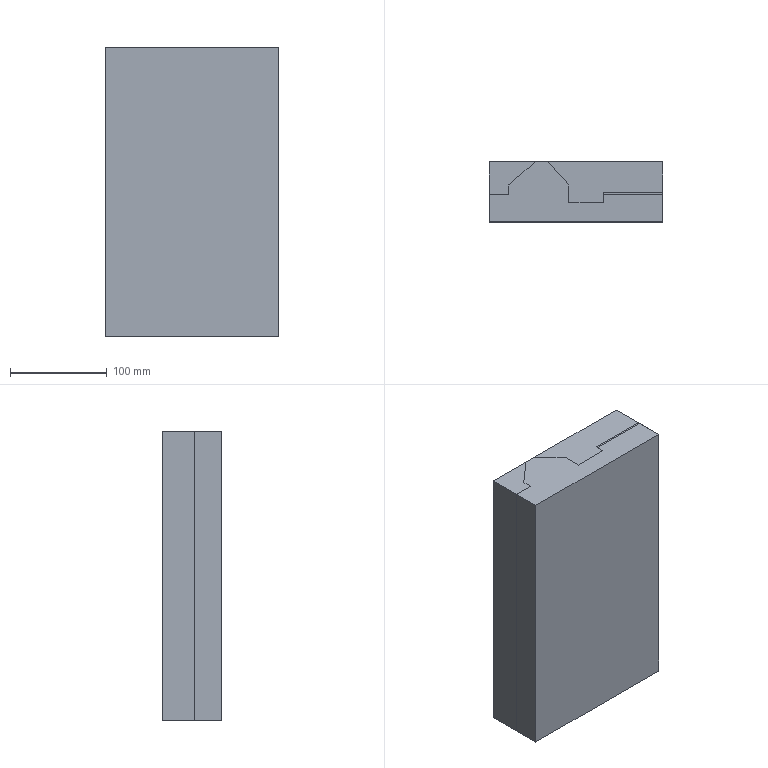NC program | NX | posted with a generic post | part box 180 x 62 x 300 mm
Lines 1 to 1029 of 29776:
N10 G17 G21 G94 G90
(型腔铣_COPY , TOOL : D50飞刀)
N12 T14 M6
N14 /M1
N16 G54
N18 G17 G0 G90 X-218.484 Y125.131 S1500 M3
N20 G43 Z20. H14
N22 Z-9.3
N24 G94 G1 Z-10.3 F2000.
N26 G3 X-181.258 Y93.895 R37.8
N28 G1 X-152.134
N30 G2 X-150. Y93.915 R113.9
N32 G1 X150.
N34 G2 X152.134 Y93.895 R113.9
N36 G1 X175.831
N38 G2 X179.344 Y92.674 R5.67 F1880.
N40 X181.345 Y89.54 R5.67 F1760.
N42 X181.5 Y88.226 R5.67 F1640.
N44 G1 Y85.763
N46 Y81.975 F1520.
N48 Y78.186 F1400.
N50 Y74.397 F1280.
N52 Y70.608 F1160.
N54 Y66.819 F1040.
N56 Y63.03 F920.
N58 Y59.242 F800.
N60 G2 X175.203 Y52.945 R6.3
N62 G1 X151.708 F2000.
N64 G3 X150. Y52.965 R72.95
N66 G1 X-150.
N68 G3 X-151.708 Y52.945 R72.95
N70 G1 X-175.201
N72 G3 X-178.934 Y51.719 R6.3 F1880.
N74 X-181.214 Y48.52 R6.3 F1760.
N76 X-181.5 Y46.646 R6.3 F1640.
N78 G1 Y44.554
N80 Y40.559 F1520.
N82 Y36.564 F1400.
N84 Y32.569 F1280.
N86 Y28.574 F1160.
N88 Y24.741 F1040.
N90 Y24.579
N92 Y24.496 F920.
N94 X-183.176 Y20.962
N96 X-184.888 Y17.352 F800.
N98 G3 X-181.5 Y11.995 R3.75
N100 G1 X-168.9
N102 X-156.3 F1040.
N104 X-151.131 F1280.
N106 G2 X-150. Y12.015 R32.
N108 G1 X-143.7
N110 X-131.1 F1520.
N112 X-118.5 F1760.
N114 X150. F2000.
N116 G2 X151.131 Y11.995 R32.
N118 G1 X181.5
N120 G3 X194.1 Y15.371 R25.2
N122 G0 Z20.
N124 X-218.449 Y125.404
N126 Z-9.6
N128 G1 Z-10.6
N130 G3 X-181.223 Y94.168 R37.8
N132 G1 X-152.129
N134 G2 X-150.013 Y94.188 R113.905
N136 G1 X150.
N138 G2 X152.134 Y94.168 R113.9
N140 G1 X175.831
N142 G2 X179.344 Y92.948 R5.67 F1880.
N144 X181.345 Y89.813 R5.67 F1760.
N146 X181.5 Y88.499 R5.67 F1640.
N148 G1 Y86.037
N150 Y82.248 F1520.
N152 Y78.459 F1400.
N154 Y74.67 F1280.
N156 Y70.881 F1160.
N158 Y67.092 F1040.
N160 Y63.304 F920.
N162 Y59.515 F800.
N164 G2 X175.203 Y53.218 R6.3
N166 G1 X151.708 F2000.
N168 G3 X150. Y53.238 R72.95
N170 G1 X-150.007
N172 G3 X-151.703 Y53.218 R72.955
N174 G1 X-175.201
N176 G3 X-178.942 Y51.987 R6.3 F1880.
N178 X-181.22 Y48.775 R6.3 F1760.
N180 X-181.5 Y46.919 R6.3 F1640.
N182 G1 Y44.798
N184 Y40.793 F1520.
N186 Y36.788 F1400.
N188 Y32.782 F1280.
N190 Y28.777 F1160.
N192 Y24.741 F1040.
N194 Y24.496 F920.
N196 X-183.098 Y21.127
N198 X-184.814 Y17.508 F800.
N200 G3 X-181.5 Y12.268 R3.668
N202 G1 X-168.9
N204 X-156.3 F1040.
N206 X-151.126 F1280.
N208 G2 X-150. Y12.288 R32.005
N210 G1 X-143.7
N212 X-131.1 F1520.
N214 X-118.5 F1760.
N216 X150. F2000.
N218 G2 X151.131 Y12.268 R32.
N220 G1 X181.5
N222 G3 X194.1 Y15.644 R25.2
N224 G0 Z20.
N226 X-218.411 Y125.678
N228 Z-9.9
N230 G1 Z-10.9
N232 G3 X-181.185 Y94.441 R37.8
N234 G1 X-152.134
N236 G2 X-150. Y94.461 R113.9
N238 G1 X150.
N240 G2 X152.134 Y94.441 R113.9
N242 G1 X175.831
N244 G2 X179.344 Y93.221 R5.67 F1880.
N246 X181.345 Y90.087 R5.67 F1760.
N248 X181.5 Y88.773 R5.67 F1640.
N250 G1 Y86.31
N252 Y82.521 F1520.
N254 Y78.733 F1400.
N256 Y74.944 F1280.
N258 Y71.155 F1160.
N260 Y67.366 F1040.
N262 Y63.577 F920.
N264 Y59.788 F800.
N266 G2 X175.203 Y53.491 R6.3
N268 G1 X151.708 F2000.
N270 G3 X150. Y53.511 R72.95
N272 G1 X-150.
N274 G3 X-151.708 Y53.491 R72.95
N276 G1 X-175.201
N278 G3 X-178.95 Y52.254 R6.3 F1880.
N280 X-181.226 Y49.029 R6.3 F1760.
N282 X-181.5 Y47.193 R6.3 F1640.
N284 G1 Y45.041
N286 Y41.026 F1520.
N288 Y37.011 F1400.
N290 Y32.996 F1280.
N292 Y28.98 F1160.
N294 Y24.965 F1040.
N296 Y24.741 F920.
N298 Y24.496
N300 X-183.019 Y21.292
N302 X-184.74 Y17.665 F800.
N304 G3 X-181.5 Y12.541 R3.586
N306 G1 X-168.9
N308 X-156.3 F1040.
N310 X-151.131 F1280.
N312 G2 X-150. Y12.561 R32.
N314 G1 X-143.7
N316 X-131.1 F1520.
N318 X-118.5 F1760.
N320 X150. F2000.
N322 G2 X151.131 Y12.541 R32.
N324 G1 X181.5
N326 G3 X194.1 Y15.918 R25.2
N328 G0 Z20.
N330 X-218.371 Y125.951
N332 Z-10.2
N334 G1 Z-11.2
N336 G3 X-181.145 Y94.715 R37.8
N338 G1 X-152.134
N340 G2 X-150. Y94.735 R113.9
N342 G1 X150.
N344 G2 X152.134 Y94.715 R113.9
N346 G1 X175.831
N348 G2 X179.344 Y93.495 R5.67 F1880.
N350 X181.345 Y90.36 R5.67 F1760.
N352 X181.5 Y89.046 R5.67 F1640.
N354 G1 Y86.584
N356 Y82.795 F1520.
N358 Y79.006 F1400.
N360 Y75.217 F1280.
N362 Y71.428 F1160.
N364 Y67.639 F1040.
N366 Y63.851 F920.
N368 Y60.062 F800.
N370 G2 X175.203 Y53.765 R6.3
N372 G1 X151.708 F2000.
N374 G3 X150. Y53.785 R72.95
N376 G1 X-150.
N378 G3 X-151.708 Y53.765 R72.95
N380 G1 X-175.201
N382 G3 X-178.958 Y52.521 R6.3 F1880.
N384 X-181.232 Y49.283 R6.3 F1760.
N386 X-181.5 Y47.466 R6.3 F1640.
N388 G1 Y45.284
N390 Y41.259 F1520.
N392 Y37.234 F1400.
N394 Y33.209 F1280.
N396 Y29.184 F1160.
N398 Y25.158 F1040.
N400 Y24.741 F920.
N402 Y24.496
N404 X-182.941 Y21.458
N406 X-184.666 Y17.821 F800.
N408 G3 X-181.5 Y12.815 R3.504
N410 G1 X-168.9
N412 X-156.3 F1040.
N414 X-151.131 F1280.
N416 G2 X-150. Y12.835 R32.
N418 G1 X-143.7
N420 X-131.1 F1520.
N422 X-118.5 F1760.
N424 X150. F2000.
N426 G2 X151.131 Y12.815 R32.
N428 G1 X181.5
N430 G3 X194.1 Y16.191 R25.2
N432 G0 Z20.
N434 X-218.328 Y126.224
N436 Z-10.5
N438 G1 Z-11.5
N440 G3 X-181.103 Y94.988 R37.8
N442 G1 X-152.134
N444 G2 X-150. Y95.008 R113.9
N446 G1 X150.
N448 G2 X152.134 Y94.988 R113.9
N450 G1 X175.831
N452 G2 X179.344 Y93.768 R5.67 F1880.
N454 X181.345 Y90.634 R5.67 F1760.
N456 X181.5 Y89.32 R5.67 F1640.
N458 G1 Y86.857
N460 Y83.068 F1520.
N462 Y79.279 F1400.
N464 Y75.491 F1280.
N466 Y71.702 F1160.
N468 Y67.913 F1040.
N470 Y64.124 F920.
N472 Y60.335 F800.
N474 G2 X175.203 Y54.038 R6.3
N476 G1 X151.708 F2000.
N478 G3 X150. Y54.058 R72.95
N480 G1 X-150.
N482 G3 X-151.708 Y54.038 R72.95
N484 G1 X-175.201
N486 G3 X-178.966 Y52.789 R6.3 F1880.
N488 X-181.238 Y49.537 R6.3 F1760.
N490 X-181.5 Y47.739 R6.3 F1640.
N492 G1 Y45.527
N494 Y41.492 F1520.
N496 Y37.457 F1400.
N498 Y33.422 F1280.
N500 Y29.387 F1160.
N502 Y25.351 F1040.
N504 Y24.741 F920.
N506 Y24.496
N508 X-182.863 Y21.623
N510 X-184.592 Y17.977 F800.
N512 G3 X-181.5 Y13.088 R3.422
N514 G1 X-168.9
N516 X-156.3 F1040.
N518 X-151.131 F1280.
N520 G2 X-150. Y13.108 R32.
N522 G1 X-143.7
N524 X-131.1 F1520.
N526 X-118.5 F1760.
N528 X150. F2000.
N530 G2 X151.131 Y13.088 R32.
N532 G1 X181.5
N534 G3 X194.1 Y16.464 R25.2
N536 G0 Z20.
N538 X-218.283 Y126.498
N540 Z-10.8
N542 G1 Z-11.8
N544 G3 X-181.057 Y95.262 R37.8
N546 G1 X-152.134
N548 G2 X-150. Y95.282 R113.9
N550 G1 X150.
N552 G2 X152.134 Y95.262 R113.9
N554 G1 X175.831
N556 G2 X179.344 Y94.041 R5.67 F1880.
N558 X181.345 Y90.907 R5.67 F1760.
N560 X181.5 Y89.593 R5.67 F1640.
N562 G1 Y87.13
N564 Y83.342 F1520.
N566 Y79.553 F1400.
N568 Y75.764 F1280.
N570 Y71.975 F1160.
N572 Y68.186 F1040.
N574 Y64.397 F920.
N576 Y60.609 F800.
N578 G2 X175.204 Y54.312 R6.3
N580 G1 X151.708 F2000.
N582 G3 X150. Y54.332 R72.95
N584 G1 X-150.
N586 G3 X-151.708 Y54.312 R72.95
N588 G1 X-175.201
N590 G3 X-178.974 Y53.056 R6.3 F1880.
N592 X-181.243 Y49.791 R6.3 F1760.
N594 X-181.5 Y48.013 R6.3 F1640.
N596 G1 Y45.771
N598 Y41.725 F1520.
N600 Y37.68 F1400.
N602 Y33.635 F1280.
N604 Y29.59 F1160.
N606 Y25.544 F1040.
N608 Y24.741 F920.
N610 Y24.496
N612 X-182.784 Y21.788
N614 X-184.518 Y18.133 F800.
N616 G3 X-181.5 Y13.362 R3.34
N618 G1 X-168.9
N620 X-156.3 F1040.
N622 X-151.131 F1280.
N624 G2 X-150. Y13.382 R32.
N626 G1 X-143.7
N628 X-131.1 F1520.
N630 X-118.5 F1760.
N632 X150. F2000.
N634 G2 X151.131 Y13.362 R32.
N636 G1 X181.5
N638 G3 X194.1 Y16.738 R25.2
N640 G0 Z20.
N642 X-218.236 Y126.771
N644 Z-11.1
N646 G1 Z-12.1
N648 G3 X-181.01 Y95.535 R37.8
N650 G1 X-152.13
N652 G2 X-150.012 Y95.555 R113.905
N654 G1 X150.
N656 G2 X152.134 Y95.535 R113.9
N658 G1 X175.831
N660 G2 X179.344 Y94.315 R5.67 F1880.
N662 X181.345 Y91.181 R5.67 F1760.
N664 X181.5 Y89.866 R5.67 F1640.
N666 G1 Y87.404
N668 Y83.615 F1520.
N670 Y79.826 F1400.
N672 Y76.037 F1280.
N674 Y72.248 F1160.
N676 Y68.46 F1040.
N678 Y64.671 F920.
N680 Y60.882 F800.
N682 G2 X175.203 Y54.585 R6.3
N684 G1 X151.708 F2000.
N686 G3 X150. Y54.605 R72.95
N688 G1 X-150.006
N690 G3 X-151.704 Y54.585 R72.955
N692 G1 X-175.201
N694 G3 X-178.982 Y53.324 R6.3 F1880.
N696 X-181.249 Y50.045 R6.3 F1760.
N698 X-181.5 Y48.286 R6.3 F1640.
N700 G1 Y46.014
N702 Y41.959 F1520.
N704 Y37.903 F1400.
N706 Y33.848 F1280.
N708 Y29.793 F1160.
N710 Y25.737 F1040.
N712 Y24.741 F920.
N714 Y24.496
N716 X-182.706 Y21.954
N718 X-184.444 Y18.289 F800.
N720 G3 X-181.5 Y13.635 R3.258
N722 G1 X-168.9
N724 X-156.3 F1040.
N726 X-151.127 F1280.
N728 G2 X-150. Y13.655 R32.005
N730 G1 X-143.7
N732 X-131.1 F1520.
N734 X-118.5 F1760.
N736 X150. F2000.
N738 G2 X151.131 Y13.635 R32.
N740 G1 X181.5
N742 G3 X194.1 Y17.011 R25.2
N744 G0 Z20.
N746 X-218.186 Y127.045
N748 Z-11.4
N750 G1 Z-12.4
N752 G3 X-180.96 Y95.808 R37.8
N754 G1 X-152.134
N756 G2 X-150. Y95.828 R113.9
N758 G1 X150.
N760 G2 X152.134 Y95.808 R113.9
N762 G1 X175.831
N764 G2 X179.344 Y94.588 R5.67 F1880.
N766 X181.345 Y91.454 R5.67 F1760.
N768 X181.5 Y90.17 R5.67 F1640.
N770 G1 Y90.
N772 Y87.677
N774 Y83.888 F1520.
N776 Y80.1 F1400.
N778 Y76.311 F1280.
N780 Y72.522 F1160.
N782 Y68.733 F1040.
N784 Y64.944 F920.
N786 Y61.155 F800.
N788 G2 X175.203 Y54.858 R6.3
N790 G1 X151.708 F2000.
N792 G3 X150. Y54.878 R72.95
N794 G1 X-150.
N796 G3 X-151.708 Y54.858 R72.95
N798 G1 X-175.201
N800 G3 X-178.99 Y53.591 R6.3 F1880.
N802 X-181.255 Y50.3 R6.3 F1760.
N804 X-181.5 Y48.56 R6.3 F1640.
N806 G1 Y46.257
N808 Y42.192 F1520.
N810 Y38.126 F1400.
N812 Y34.061 F1280.
N814 Y29.996 F1160.
N816 Y25.93 F1040.
N818 Y24.741 F920.
N820 Y24.496
N822 X-182.627 Y22.119
N824 X-184.369 Y18.446 F800.
N826 G3 X-181.5 Y13.908 R3.176
N828 G1 X-168.9
N830 X-156.3 F1040.
N832 X-151.131 F1280.
N834 G2 X-150. Y13.928 R32.
N836 G1 X-143.7
N838 X-131.1 F1520.
N840 X-118.5 F1760.
N842 X150. F2000.
N844 G2 X151.131 Y13.908 R32.
N846 G1 X181.5
N848 G3 X194.1 Y17.285 R25.2
N850 G0 Z20.
N852 X-218.133 Y127.318
N854 Z-11.7
N856 G1 Z-12.7
N858 G3 X-180.907 Y96.082 R37.8
N860 G1 X-152.134
N862 G2 X-150. Y96.102 R113.9
N864 G1 X150.
N866 G2 X152.134 Y96.082 R113.9
N868 G1 X175.828
N870 G2 X179.341 Y94.862 R5.67 F1880.
N872 X181.342 Y91.727 R5.67 F1760.
N874 X181.496 Y90.504 R5.67 F1640.
N876 X181.5 Y90. R31.5
N878 G1 Y87.951
N880 Y84.162 F1520.
N882 Y80.373 F1400.
N884 Y76.584 F1280.
N886 Y72.795 F1160.
N888 Y69.006 F1040.
N890 Y65.218 F920.
N892 Y61.429 F800.
N894 G2 X175.203 Y55.132 R6.3
N896 G1 X151.708 F2000.
N898 G3 X150. Y55.152 R72.95
N900 G1 X-150.
N902 G3 X-151.708 Y55.132 R72.95
N904 G1 X-175.201
N906 G3 X-178.998 Y53.858 R6.3 F1880.
N908 X-181.26 Y50.554 R6.3 F1760.
N910 X-181.5 Y48.833 R6.3 F1640.
N912 G1 Y46.5
N914 Y42.425 F1520.
N916 Y38.35 F1400.
N918 Y34.274 F1280.
N920 Y30.199 F1160.
N922 Y26.123 F1040.
N924 Y24.741 F920.
N926 Y24.496
N928 X-182.549 Y22.284
N930 X-184.295 Y18.602 F800.
N932 G3 X-181.5 Y14.182 R3.094
N934 G1 X-168.9
N936 X-156.3 F1040.
N938 X-151.131 F1280.
N940 G2 X-150. Y14.202 R32.
N942 G1 X-143.7
N944 X-131.1 F1520.
N946 X-118.5 F1760.
N948 X150. F2000.
N950 G2 X151.131 Y14.182 R32.
N952 G1 X181.5
N954 G3 X194.1 Y17.558 R25.2
N956 G0 Z20.
N958 X-218.078 Y127.591
N960 Z-12.
N962 G1 Z-13.
N964 G3 X-180.852 Y96.355 R37.8
N966 G1 X-152.134
N968 G2 X-150. Y96.375 R113.9
N970 G1 X150.
N972 G2 X152.134 Y96.355 R113.9
N974 G1 X175.822
N976 G2 X179.335 Y95.135 R5.67 F1880.
N978 X181.336 Y92.001 R5.67 F1760.
N980 X181.489 Y90.837 R5.67 F1640.
N982 X181.5 Y90. R31.5
N984 G1 Y88.224
N986 Y84.435 F1520.
N988 Y80.646 F1400.
N990 Y76.858 F1280.
N992 Y73.069 F1160.
N994 Y69.28 F1040.
N996 Y65.491 F920.
N998 Y61.702 F800.
N1000 G2 X175.204 Y55.405 R6.3
N1002 G1 X151.708 F2000.
N1004 G3 X150. Y55.425 R72.95
N1006 G1 X-150.
N1008 G3 X-151.708 Y55.405 R72.95
N1010 G1 X-175.201
N1012 G3 X-179.006 Y54.126 R6.3 F1880.
N1014 X-181.266 Y50.808 R6.3 F1760.
N1016 X-181.5 Y49.107 R6.3 F1640.
N1018 G1 Y46.744
N1020 Y42.658 F1520.
N1022 Y38.573 F1400.
N1024 Y34.487 F1280.
N1026 Y30.402 F1160.
N1028 Y26.316 F1040.
N1030 Y24.741 F920.
N1032 Y24.496
N1034 X-182.47 Y22.449
N1036 X-184.221 Y18.758 F800.
N1038 G3 X-181.5 Y14.455 R3.012
N1040 G1 X-168.9
N1042 X-156.3 F1040.
N1044 X-151.131 F1280.
N1046 G2 X-150. Y14.475 R32.
N1048 G1 X-143.7
N1050 X-131.1 F1520.
N1052 X-118.5 F1760.
N1054 X150. F2000.
N1056 G2 X151.131 Y14.455 R32.
N1058 G1 X181.5
N1060 G3 X194.1 Y17.831 R25.2
N1062 G0 Z20.
N1064 X-218.02 Y127.865
N1066 Z-12.3
N1068 G1 Z-13.3
N1070 G3 X-180.795 Y96.629 R37.8
N1072 G1 X-152.134
N1074 G2 X-150. Y96.649 R113.9
N1076 G1 X150.
N1078 G2 X152.134 Y96.629 R113.9
N1080 G1 X175.199
N1082 G2 X178.793 Y95.502 R6.3 F1880.
N1084 X181.102 Y92.527 R6.3 F1760.
N1086 X181.497 Y90.412 R6.3 F1640.
N1088 X181.5 Y90. R31.5
N1090 G1 Y88.749
N1092 Y84.924 F1520.
N1094 Y81.1 F1400.
N1096 Y77.275 F1280.
N1098 Y73.45 F1160.
N1100 Y69.625 F1040.
N1102 Y65.8 F920.
N1104 Y61.976 F800.
N1106 G2 X175.203 Y55.679 R6.3
N1108 G1 X151.708 F2000.
N1110 G3 X150. Y55.699 R72.95
N1112 G1 X-150.
N1114 G3 X-151.708 Y55.679 R72.95
N1116 G1 X-175.201
N1118 G3 X-179.014 Y54.393 R6.3 F1880.
N1120 X-181.271 Y51.062 R6.3 F1760.
N1122 X-181.5 Y49.38 R6.3 F1640.
N1124 G1 Y46.987
N1126 Y42.891 F1520.
N1128 Y38.796 F1400.
N1130 Y34.7 F1280.
N1132 Y30.605 F1160.
N1134 Y26.509 F1040.
N1136 Y24.741 F920.
N1138 Y24.496
N1140 X-182.392 Y22.615
N1142 X-184.147 Y18.914 F800.
N1144 G3 X-181.5 Y14.729 R2.93
N1146 G1 X-168.9
N1148 X-156.3 F1040.
N1150 X-151.131 F1280.
N1152 G2 X-150. Y14.749 R32.
N1154 G1 X-143.7
N1156 X-131.1 F1520.
N1158 X-118.5 F1760.
N1160 X150. F2000.
N1162 G2 X151.131 Y14.729 R32.
N1164 G1 X181.5
N1166 G3 X194.1 Y18.105 R25.2
N1168 G0 Z20.
N1170 X-217.96 Y128.138
N1172 Z-12.6
N1174 G1 Z-13.6
N1176 G3 X-180.735 Y96.902 R37.8
N1178 G1 X-152.134
N1180 G2 X-150. Y96.922 R113.9
N1182 G1 X150.
N1184 G2 X152.134 Y96.902 R113.9
N1186 G1 X175.194
N1188 G2 X178.788 Y95.776 R6.3 F1880.
N1190 X181.097 Y92.8 R6.3 F1760.
N1192 X181.491 Y90.754 R6.3 F1640.
N1194 X181.5 Y90. R31.5
N1196 G1 Y89.918
N1198 Y89.023
N1200 Y85.198 F1520.
N1202 Y81.373 F1400.
N1204 Y77.548 F1280.
N1206 Y73.723 F1160.
N1208 Y69.899 F1040.
N1210 Y66.074 F920.
N1212 Y62.249 F800.
N1214 G2 X175.203 Y55.952 R6.3
N1216 G1 X151.708 F2000.
N1218 G3 X150. Y55.972 R72.95
N1220 G1 X-150.
N1222 G3 X-151.708 Y55.952 R72.95
N1224 G1 X-175.201
N1226 G3 X-179.022 Y54.66 R6.3 F1880.
N1228 X-181.276 Y51.316 R6.3 F1760.
N1230 X-181.5 Y49.653 R6.3 F1640.
N1232 G1 Y47.23
N1234 Y43.125 F1520.
N1236 Y39.019 F1400.
N1238 Y34.914 F1280.
N1240 Y30.808 F1160.
N1242 Y26.702 F1040.
N1244 Y24.741 F920.
N1246 Y24.496
N1248 X-182.314 Y22.78
N1250 X-184.073 Y19.071 F800.
N1252 G3 X-181.5 Y15.002 R2.848
N1254 G1 X-168.9
N1256 X-156.3 F1040.
N1258 X-151.131 F1280.
N1260 G2 X-150. Y15.022 R32.
N1262 G1 X-143.7
N1264 X-131.1 F1520.
N1266 X-118.5 F1760.
N1268 X150. F2000.
N1270 G2 X151.131 Y15.002 R32.
N1272 G1 X181.5
N1274 G3 X194.1 Y18.378 R25.2
N1276 G0 Z20.
N1278 X-217.898 Y128.412
N1280 Z-12.9
N1282 G1 Z-13.9
N1284 G3 X-180.672 Y97.175 R37.8
N1286 G1 X-152.13
N1288 G2 X-150.012 Y97.195 R113.905
N1290 G1 X150.013
N1292 G2 X152.13 Y97.175 R113.905
N1294 G1 X175.186
N1296 G2 X178.78 Y96.049 R6.3 F1880.
N1298 X181.089 Y93.073 R6.3 F1760.
N1300 X181.481 Y91.096 R6.3 F1640.
N1302 X181.5 Y90. R31.5
N1304 G1 Y89.918
N1306 Y89.296
N1308 Y85.471 F1520.
N1310 Y81.646 F1400.
N1312 Y77.822 F1280.
N1314 Y73.997 F1160.
N1316 Y70.172 F1040.
N1318 Y66.347 F920.
N1320 Y62.522 F800.
N1322 G2 X175.203 Y56.225 R6.3
N1324 G1 X151.703 F2000.
N1326 G3 X150.006 Y56.245 R72.955
N1328 G1 X-150.006
N1330 G3 X-151.704 Y56.225 R72.955
N1332 G1 X-175.201
N1334 G3 X-179.03 Y54.928 R6.3 F1880.
N1336 X-181.282 Y51.57 R6.3 F1760.
N1338 X-181.5 Y49.927 R6.3 F1640.
N1340 G1 Y47.473
N1342 Y43.358 F1520.
N1344 Y39.242 F1400.
N1346 Y35.127 F1280.
N1348 Y31.011 F1160.
N1350 Y26.895 F1040.
N1352 Y24.741 F920.
N1354 Y24.496
N1356 X-182.235 Y22.945
N1358 X-183.999 Y19.227 F800.
N1360 G3 X-181.5 Y15.275 R2.766
N1362 G1 X-168.9
N1364 X-156.3 F1040.
N1366 X-151.127 F1280.
N1368 G2 X-150. Y15.295 R32.005
N1370 G1 X-143.7
N1372 X-131.1 F1520.
N1374 X-118.5 F1760.
N1376 X150. F2000.
N1378 G2 X151.126 Y15.275 R32.005
N1380 G1 X181.5
N1382 G3 X194.1 Y18.652 R25.2
N1384 G0 Z20.
N1386 X-217.832 Y128.685
N1388 Z-13.2
N1390 G1 Z-14.2
N1392 G3 X-180.607 Y97.449 R37.8
N1394 G1 X-152.134
N1396 G2 X-150. Y97.469 R113.9
N1398 G1 X150.
N1400 G2 X152.134 Y97.449 R113.9
N1402 G1 X175.175
N1404 G2 X178.769 Y96.322 R6.3 F1880.
N1406 X181.078 Y93.347 R6.3 F1760.
N1408 X181.467 Y91.437 R6.3 F1640.
N1410 X181.5 Y90. R31.5
N1412 G1 Y89.57
N1414 Y85.745 F1520.
N1416 Y81.92 F1400.
N1418 Y78.095 F1280.
N1420 Y74.27 F1160.
N1422 Y70.445 F1040.
N1424 Y66.621 F920.
N1426 Y62.796 F800.
N1428 G2 X175.203 Y56.499 R6.3
N1430 G1 X151.708 F2000.
N1432 G3 X150. Y56.519 R72.95
N1434 G1 X-150.
N1436 G3 X-151.708 Y56.499 R72.95
N1438 G1 X-175.201
N1440 G3 X-179.038 Y55.195 R6.3 F1880.
N1442 X-181.287 Y51.824 R6.3 F1760.
N1444 X-181.5 Y50.2 R6.3 F1640.
N1446 G1 Y47.717
N1448 Y43.591 F1520.
N1450 Y39.465 F1400.
N1452 Y35.34 F1280.
N1454 Y31.214 F1160.
N1456 Y27.088 F1040.
N1458 Y24.741 F920.
N1460 Y24.496
N1462 X-182.157 Y23.111
N1464 X-183.925 Y19.383 F800.
N1466 G3 X-181.5 Y15.549 R2.684
N1468 G1 X-168.9
N1470 X-156.3 F1040.
N1472 X-151.131 F1280.
N1474 G2 X-150. Y15.569 R32.
N1476 G1 X-143.7
N1478 X-131.1 F1520.
N1480 X-118.5 F1760.
N1482 X150. F2000.
N1484 G2 X151.131 Y15.549 R32.
N1486 G1 X181.5
N1488 G3 X194.1 Y18.925 R25.2
N1490 G0 Z20.
N1492 X-217.765 Y128.958
N1494 Z-13.5
N1496 G1 Z-14.5
N1498 G3 X-180.539 Y97.722 R37.8
N1500 G1 X-152.134
N1502 G2 X-150. Y97.742 R113.9
N1504 G1 X150.
N1506 G2 X152.134 Y97.722 R113.9
N1508 G1 X175.161
N1510 G2 X178.755 Y96.596 R6.3 F1880.
N1512 X181.064 Y93.62 R6.3 F1760.
N1514 X181.45 Y91.779 R6.3 F1640.
N1516 X181.5 Y90. R31.5
N1518 G1 Y89.918
N1520 Y89.843
N1522 Y86.018 F1520.
N1524 Y82.194 F1400.
N1526 Y78.369 F1280.
N1528 Y74.544 F1160.
N1530 Y70.719 F1040.
N1532 Y66.894 F920.
N1534 Y63.069 F800.
N1536 G2 X175.203 Y56.772 R6.3
N1538 G1 X151.708 F2000.
N1540 G3 X150. Y56.792 R72.95
N1542 G1 X-150.
N1544 G3 X-151.708 Y56.772 R72.95
N1546 G1 X-175.201
N1548 G3 X-179.046 Y55.462 R6.3 F1880.
N1550 X-181.292 Y52.078 R6.3 F1760.
N1552 X-181.5 Y50.473 R6.3 F1640.
N1554 G1 Y47.96
N1556 Y43.824 F1520.
N1558 Y39.689 F1400.
N1560 Y35.553 F1280.
N1562 Y31.417 F1160.
N1564 Y27.282 F1040.
N1566 Y24.741 F920.
N1568 Y24.496
N1570 X-182.078 Y23.276
N1572 X-183.851 Y19.539 F800.
N1574 G3 X-181.5 Y15.822 R2.602
N1576 G1 X-168.9
N1578 X-156.3 F1040.
N1580 X-151.131 F1280.
N1582 G2 X-150. Y15.842 R32.
N1584 G1 X-143.7
N1586 X-131.1 F1520.
N1588 X-118.5 F1760.
N1590 X150. F2000.
N1592 G2 X151.131 Y15.822 R32.
N1594 G1 X181.5
N1596 G3 X194.1 Y19.198 R25.2
N1598 G0 Z20.
N1600 X-217.694 Y129.232
N1602 Z-13.8
N1604 G1 Z-14.8
N1606 G3 X-180.468 Y97.996 R37.8
N1608 G1 X-152.134
N1610 G2 X-150. Y98.016 R113.9
N1612 G1 X150.
N1614 G2 X152.134 Y97.996 R113.9
N1616 G1 X175.144
N1618 G2 X178.738 Y96.869 R6.3 F1880.
N1620 X181.047 Y93.894 R6.3 F1760.
N1622 X181.429 Y92.121 R6.3 F1640.
N1624 X181.5 Y90.117 R31.5
N1626 G1 Y90. F1520.
N1628 Y86.292
N1630 Y82.467 F1400.
N1632 Y78.642 F1280.
N1634 Y74.817 F1160.
N1636 Y70.992 F1040.
N1638 Y67.168 F920.
N1640 Y63.343 F800.
N1642 G2 X175.203 Y57.046 R6.3
N1644 G1 X151.708 F2000.
N1646 G3 X150. Y57.066 R72.95
N1648 G1 X-150.
N1650 G3 X-151.708 Y57.046 R72.95
N1652 G1 X-175.201
N1654 G3 X-179.054 Y55.729 R6.3 F1880.
N1656 X-181.297 Y52.332 R6.3 F1760.
N1658 X-181.5 Y50.747 R6.3 F1640.
N1660 G1 Y48.203
N1662 Y44.058 F1520.
N1664 Y39.912 F1400.
N1666 Y35.766 F1280.
N1668 Y31.62 F1160.
N1670 Y27.475 F1040.
N1672 Y24.741 F920.
N1674 Y24.496
N1676 X-182. Y23.441
N1678 X-183.777 Y19.696 F800.
N1680 G3 X-181.5 Y16.096 R2.52
N1682 G1 X-168.9
N1684 X-156.3 F1040.
N1686 X-151.131 F1280.
N1688 G2 X-150. Y16.116 R32.
N1690 G1 X-143.7
N1692 X-131.1 F1520.
N1694 X-118.5 F1760.
N1696 X150. F2000.
N1698 G2 X151.131 Y16.096 R32.
N1700 G1 X181.5
N1702 G3 X194.1 Y19.472 R25.2
N1704 G0 Z20.
N1706 X-217.621 Y129.505
N1708 Z-14.1
N1710 G1 Z-15.1
N1712 G3 X-180.395 Y98.269 R37.8
N1714 G1 X-152.134
N1716 G2 X-150. Y98.289 R113.9
N1718 G1 X150.
N1720 G2 X152.134 Y98.269 R113.9
N1722 G1 X175.124
N1724 G2 X178.718 Y97.142 R6.3 F1880.
N1726 X181.027 Y94.167 R6.3 F1760.
N1728 X181.404 Y92.463 R6.3 F1640.
N1730 X181.498 Y90.391 R31.5
N1732 X181.5 Y90. R31.5 F1520.
N1734 G1 Y89.918
N1736 Y86.566
N1738 Y82.741 F1400.
N1740 Y78.916 F1280.
N1742 Y75.091 F1160.
N1744 Y71.266 F1040.
N1746 Y67.441 F920.
N1748 Y63.616 F800.
N1750 G2 X175.203 Y57.319 R6.3
N1752 G1 X151.708 F2000.
N1754 G3 X150. Y57.339 R72.95
N1756 G1 X-150.
N1758 G3 X-151.708 Y57.319 R72.95
N1760 G1 X-175.201
N1762 G3 X-179.062 Y55.997 R6.3 F1880.
N1764 X-181.302 Y52.586 R6.3 F1760.
N1766 X-181.5 Y51.02 R6.3 F1640.
N1768 G1 Y48.446
N1770 Y44.291 F1520.
N1772 Y40.135 F1400.
N1774 Y35.979 F1280.
N1776 Y31.823 F1160.
N1778 Y27.668 F1040.
N1780 Y24.741 F920.
N1782 Y24.496
N1784 X-181.922 Y23.607
N1786 X-183.703 Y19.852 F800.
N1788 G3 X-181.5 Y16.369 R2.438
N1790 G1 X-168.9
N1792 X-156.3 F1040.
N1794 X-151.131 F1280.
N1796 G2 X-150. Y16.389 R32.
N1798 G1 X-143.7
N1800 X-131.1 F1520.
N1802 X-118.5 F1760.
N1804 X150. F2000.
N1806 G2 X151.131 Y16.369 R32.
N1808 G1 X181.5
N1810 G3 X194.1 Y19.745 R25.2
N1812 G0 Z20.
N1814 X-217.545 Y129.779
N1816 Z-14.4
N1818 G1 Z-15.4
N1820 G3 X-180.32 Y98.542 R37.8
N1822 G1 X-152.134
N1824 G2 X-150.006 Y98.562 R113.9
N1826 G1 X150.
N1828 G2 X152.134 Y98.542 R113.9
N1830 G1 X175.101
N1832 G2 X178.695 Y97.416 R6.3 F1880.
N1834 X181.004 Y94.44 R6.3 F1760.
N1836 X181.375 Y92.805 R6.3 F1640.
N1838 X181.493 Y90.665 R31.5
N1840 X181.5 Y90. R31.5 F1520.
N1842 G1 Y86.84
N1844 Y83.015 F1400.
N1846 Y79.19 F1280.
N1848 Y75.365 F1160.
N1850 Y71.54 F1040.
N1852 Y67.714 F920.
N1854 Y63.889 F800.
N1856 G2 X175.203 Y57.592 R6.3
N1858 G1 X151.708 F2000.
N1860 G3 X150. Y57.612 R72.95
N1862 G1 X-150.
N1864 G3 X-151.708 Y57.592 R72.95
N1866 G1 X-175.201
N1868 G3 X-179.07 Y56.264 R6.3 F1880.
N1870 X-181.307 Y52.84 R6.3 F1760.
N1872 X-181.5 Y51.294 R6.3 F1640.
N1874 G1 Y48.69
N1876 Y44.524 F1520.
N1878 Y40.358 F1400.
N1880 Y36.192 F1280.
N1882 Y32.026 F1160.
N1884 Y27.861 F1040.
N1886 Y24.741 F920.
N1888 Y24.496
N1890 X-181.843 Y23.772
N1892 X-183.628 Y20.008 F800.
N1894 G3 X-181.5 Y16.642 R2.356
N1896 G1 X-168.9
N1898 X-156.3 F1040.
N1900 X-151.131 F1280.
N1902 G2 X-150. Y16.662 R32.
N1904 G1 X-143.7
N1906 X-131.1 F1520.
N1908 X-118.5 F1760.
N1910 X150. F2000.
N1912 G2 X151.131 Y16.642 R32.
N1914 G1 X181.5
N1916 G3 X194.1 Y20.019 R25.2
N1918 G0 Z20.
N1920 X-217.467 Y130.052
N1922 Z-14.7
N1924 G1 Z-15.7
N1926 G3 X-180.241 Y98.816 R37.8
N1928 G1 X-152.13
N1930 G2 X-150.012 Y98.836 R113.905
N1932 G1 X150.013
N1934 G2 X152.13 Y98.816 R113.905
N1936 G1 X175.075
N1938 G2 X178.67 Y97.689 R6.3 F1880.
N1940 X180.979 Y94.713 R6.3 F1760.
N1942 X181.342 Y93.146 R6.3 F1640.
N1944 X181.486 Y90.939 R31.5
N1946 X181.5 Y90. R31.5 F1520.
N1948 G1 Y87.114
N1950 Y83.289 F1400.
N1952 Y79.463 F1280.
N1954 Y75.638 F1160.
N1956 Y71.813 F1040.
N1958 Y67.988 F920.
N1960 Y64.163 F800.
N1962 G2 X175.203 Y57.866 R6.3
N1964 G1 X151.703 F2000.
N1966 G3 X150.006 Y57.886 R72.955
N1968 G1 X-150.006
N1970 G3 X-151.703 Y57.866 R72.955
N1972 G1 X-175.201
N1974 G3 X-179.078 Y56.531 R6.3 F1880.
N1976 X-181.312 Y53.093 R6.3 F1760.
N1978 X-181.5 Y51.567 R6.3 F1640.
N1980 G1 Y48.933
N1982 Y44.757 F1520.
N1984 Y40.581 F1400.
N1986 Y36.405 F1280.
N1988 Y32.229 F1160.
N1990 Y28.054 F1040.
N1992 Y24.741 F920.
N1994 Y24.496
N1996 X-181.765 Y23.937
N1998 X-183.554 Y20.164 F800.
N2000 G3 X-181.5 Y16.916 R2.274
N2002 G1 X-168.9
N2004 X-156.3 F1040.
N2006 X-151.127 F1280.
N2008 G2 X-150. Y16.936 R32.005
N2010 G1 X-143.7
N2012 X-131.1 F1520.
N2014 X-118.5 F1760.
N2016 X150. F2000.
N2018 G2 X151.126 Y16.916 R32.005
N2020 G1 X181.5
N2022 G3 X194.1 Y20.292 R25.2
N2024 G0 Z20.
N2026 X-217.386 Y130.325
N2028 Z-15.
N2030 G1 Z-16.
N2032 G3 X-180.16 Y99.089 R37.8
N2034 G1 X-152.134
N2036 G2 X-150. Y99.109 R113.9
N2038 G1 X150.
N2040 G2 X152.134 Y99.089 R113.9
N2042 G1 X175.046
N2044 G2 X178.641 Y97.963 R6.3 F1880.
N2046 X180.95 Y94.986 R6.3 F1760.
N2048 X181.306 Y93.488 R6.3 F1640.
N2050 X181.477 Y91.213 R31.5
N2052 X181.5 Y90. R31.5 F1520.
N2054 G1 Y89.918
N2056 Y87.388